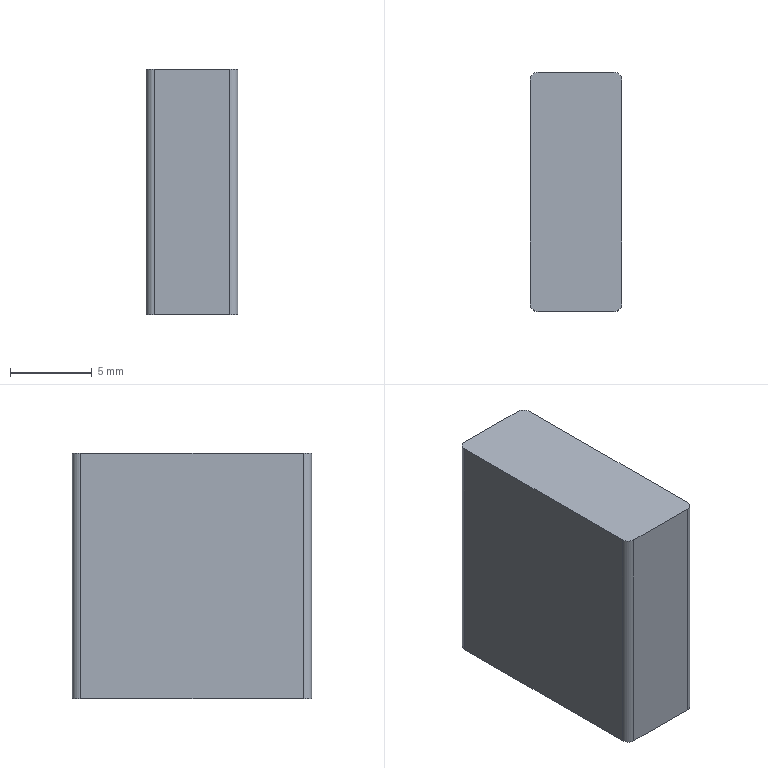Part | NX | features BREP 1 | 1 solid | 10 faces | box 5.6 x 14.6 x 15 mm | volume 1223 mm3 | plane 6 | cylinder 4 | commonest cylinder face diameters 1 x4
STEP:
#1=CARTESIAN_POINT('',(-2.3,7.3,-25.6));
#2=VERTEX_POINT('',#1);
#3=CARTESIAN_POINT('',(-2.8,6.8,-25.6));
#4=VERTEX_POINT('',#3);
#5=CARTESIAN_POINT('',(-2.3,6.8,-25.6));
#6=DIRECTION('',(0.,0.,1.));
#7=DIRECTION('',(1.,0.,0.));
#8=AXIS2_PLACEMENT_3D('',#5,#6,#7);
#9=CIRCLE('',#8,0.5);
#10=EDGE_CURVE('',#2,#4,#9,.T.);
#11=ORIENTED_EDGE('',*,*,#10,.F.);
#12=CARTESIAN_POINT('',(-2.3,7.3,-40.6));
#13=VERTEX_POINT('',#12);
#14=CARTESIAN_POINT('',(-2.3,7.3,-40.6));
#15=DIRECTION('',(0.,0.,1.));
#16=VECTOR('',#15,1000.);
#17=LINE('',#14,#16);
#18=EDGE_CURVE('',#13,#2,#17,.T.);
#19=ORIENTED_EDGE('',*,*,#18,.F.);
#20=CARTESIAN_POINT('',(-2.8,6.8,-40.6));
#21=VERTEX_POINT('',#20);
#22=CARTESIAN_POINT('',(-2.3,6.8,-40.6));
#23=DIRECTION('',(0.,0.,1.));
#24=DIRECTION('',(1.,0.,0.));
#25=AXIS2_PLACEMENT_3D('',#22,#23,#24);
#26=CIRCLE('',#25,0.5);
#27=EDGE_CURVE('',#13,#21,#26,.T.);
#28=ORIENTED_EDGE('',*,*,#27,.T.);
#29=CARTESIAN_POINT('',(-2.8,6.8,-40.6));
#30=DIRECTION('',(0.,0.,1.));
#31=VECTOR('',#30,1000.);
#32=LINE('',#29,#31);
#33=EDGE_CURVE('',#21,#4,#32,.T.);
#34=ORIENTED_EDGE('',*,*,#33,.T.);
#35=EDGE_LOOP('',(#11,#19,#28,#34));
#36=FACE_BOUND('',#35,.T.);
#37=CARTESIAN_POINT('',(-2.3,6.8,-40.6));
#38=DIRECTION('',(0.,0.,1.));
#39=DIRECTION('',(-1.,0.,0.));
#40=AXIS2_PLACEMENT_3D('',#37,#38,#39);
#41=CYLINDRICAL_SURFACE('',#40,0.5);
#42=ADVANCED_FACE('',(#36),#41,.T.);
#43=CARTESIAN_POINT('',(-2.8,-6.8,-25.6));
#44=VERTEX_POINT('',#43);
#45=CARTESIAN_POINT('',(-2.8,-6.8,-25.6));
#46=DIRECTION('',(0.,1.,0.));
#47=VECTOR('',#46,1000.);
#48=LINE('',#45,#47);
#49=EDGE_CURVE('',#44,#4,#48,.T.);
#50=ORIENTED_EDGE('',*,*,#49,.T.);
#51=ORIENTED_EDGE('',*,*,#33,.F.);
#52=CARTESIAN_POINT('',(-2.8,-6.8,-40.6));
#53=VERTEX_POINT('',#52);
#54=CARTESIAN_POINT('',(-2.8,-6.8,-40.6));
#55=DIRECTION('',(0.,1.,0.));
#56=VECTOR('',#55,1000.);
#57=LINE('',#54,#56);
#58=EDGE_CURVE('',#53,#21,#57,.T.);
#59=ORIENTED_EDGE('',*,*,#58,.F.);
#60=CARTESIAN_POINT('',(-2.8,-6.8,-40.6));
#61=DIRECTION('',(0.,0.,1.));
#62=VECTOR('',#61,1000.);
#63=LINE('',#60,#62);
#64=EDGE_CURVE('',#53,#44,#63,.T.);
#65=ORIENTED_EDGE('',*,*,#64,.T.);
#66=EDGE_LOOP('',(#50,#51,#59,#65));
#67=FACE_BOUND('',#66,.T.);
#68=CARTESIAN_POINT('',(-2.8,-6.8,-40.6));
#69=DIRECTION('',(1.,0.,0.));
#70=DIRECTION('',(0.,-1.,0.));
#71=AXIS2_PLACEMENT_3D('',#68,#69,#70);
#72=PLANE('',#71);
#73=ADVANCED_FACE('',(#67),#72,.F.);
#74=CARTESIAN_POINT('',(-2.3,-7.3,-25.6));
#75=VERTEX_POINT('',#74);
#76=CARTESIAN_POINT('',(-2.3,-6.8,-25.6));
#77=DIRECTION('',(0.,0.,1.));
#78=DIRECTION('',(1.,0.,0.));
#79=AXIS2_PLACEMENT_3D('',#76,#77,#78);
#80=CIRCLE('',#79,0.5);
#81=EDGE_CURVE('',#44,#75,#80,.T.);
#82=ORIENTED_EDGE('',*,*,#81,.F.);
#83=ORIENTED_EDGE('',*,*,#64,.F.);
#84=CARTESIAN_POINT('',(-2.3,-7.3,-40.6));
#85=VERTEX_POINT('',#84);
#86=CARTESIAN_POINT('',(-2.3,-6.8,-40.6));
#87=DIRECTION('',(0.,0.,1.));
#88=DIRECTION('',(1.,0.,0.));
#89=AXIS2_PLACEMENT_3D('',#86,#87,#88);
#90=CIRCLE('',#89,0.5);
#91=EDGE_CURVE('',#53,#85,#90,.T.);
#92=ORIENTED_EDGE('',*,*,#91,.T.);
#93=CARTESIAN_POINT('',(-2.3,-7.3,-40.6));
#94=DIRECTION('',(0.,0.,1.));
#95=VECTOR('',#94,1000.);
#96=LINE('',#93,#95);
#97=EDGE_CURVE('',#85,#75,#96,.T.);
#98=ORIENTED_EDGE('',*,*,#97,.T.);
#99=EDGE_LOOP('',(#82,#83,#92,#98));
#100=FACE_BOUND('',#99,.T.);
#101=CARTESIAN_POINT('',(-2.3,-6.8,-40.6));
#102=DIRECTION('',(0.,0.,1.));
#103=DIRECTION('',(-1.,0.,0.));
#104=AXIS2_PLACEMENT_3D('',#101,#102,#103);
#105=CYLINDRICAL_SURFACE('',#104,0.5);
#106=ADVANCED_FACE('',(#100),#105,.T.);
#107=CARTESIAN_POINT('',(2.3,-7.3,-25.6));
#108=VERTEX_POINT('',#107);
#109=CARTESIAN_POINT('',(2.3,-7.3,-25.6));
#110=DIRECTION('',(-1.,0.,0.));
#111=VECTOR('',#110,1000.);
#112=LINE('',#109,#111);
#113=EDGE_CURVE('',#108,#75,#112,.T.);
#114=ORIENTED_EDGE('',*,*,#113,.T.);
#115=ORIENTED_EDGE('',*,*,#97,.F.);
#116=CARTESIAN_POINT('',(2.3,-7.3,-40.6));
#117=VERTEX_POINT('',#116);
#118=CARTESIAN_POINT('',(2.3,-7.3,-40.6));
#119=DIRECTION('',(-1.,0.,0.));
#120=VECTOR('',#119,1000.);
#121=LINE('',#118,#120);
#122=EDGE_CURVE('',#117,#85,#121,.T.);
#123=ORIENTED_EDGE('',*,*,#122,.F.);
#124=CARTESIAN_POINT('',(2.3,-7.3,-40.6));
#125=DIRECTION('',(0.,0.,1.));
#126=VECTOR('',#125,1000.);
#127=LINE('',#124,#126);
#128=EDGE_CURVE('',#117,#108,#127,.T.);
#129=ORIENTED_EDGE('',*,*,#128,.T.);
#130=EDGE_LOOP('',(#114,#115,#123,#129));
#131=FACE_BOUND('',#130,.T.);
#132=CARTESIAN_POINT('',(2.3,-7.3,-40.6));
#133=DIRECTION('',(0.,1.,0.));
#134=DIRECTION('',(0.,0.,-1.));
#135=AXIS2_PLACEMENT_3D('',#132,#133,#134);
#136=PLANE('',#135);
#137=ADVANCED_FACE('',(#131),#136,.F.);
#138=CARTESIAN_POINT('',(2.8,-6.8,-25.6));
#139=VERTEX_POINT('',#138);
#140=CARTESIAN_POINT('',(2.3,-6.8,-25.6));
#141=DIRECTION('',(0.,0.,1.));
#142=DIRECTION('',(1.,0.,0.));
#143=AXIS2_PLACEMENT_3D('',#140,#141,#142);
#144=CIRCLE('',#143,0.5);
#145=EDGE_CURVE('',#108,#139,#144,.T.);
#146=ORIENTED_EDGE('',*,*,#145,.F.);
#147=ORIENTED_EDGE('',*,*,#128,.F.);
#148=CARTESIAN_POINT('',(2.8,-6.8,-40.6));
#149=VERTEX_POINT('',#148);
#150=CARTESIAN_POINT('',(2.3,-6.8,-40.6));
#151=DIRECTION('',(0.,0.,1.));
#152=DIRECTION('',(1.,0.,0.));
#153=AXIS2_PLACEMENT_3D('',#150,#151,#152);
#154=CIRCLE('',#153,0.5);
#155=EDGE_CURVE('',#117,#149,#154,.T.);
#156=ORIENTED_EDGE('',*,*,#155,.T.);
#157=CARTESIAN_POINT('',(2.8,-6.8,-40.6));
#158=DIRECTION('',(0.,0.,1.));
#159=VECTOR('',#158,1000.);
#160=LINE('',#157,#159);
#161=EDGE_CURVE('',#149,#139,#160,.T.);
#162=ORIENTED_EDGE('',*,*,#161,.T.);
#163=EDGE_LOOP('',(#146,#147,#156,#162));
#164=FACE_BOUND('',#163,.T.);
#165=CARTESIAN_POINT('',(2.3,-6.8,-40.6));
#166=DIRECTION('',(0.,0.,1.));
#167=DIRECTION('',(-1.,0.,0.));
#168=AXIS2_PLACEMENT_3D('',#165,#166,#167);
#169=CYLINDRICAL_SURFACE('',#168,0.5);
#170=ADVANCED_FACE('',(#164),#169,.T.);
#171=CARTESIAN_POINT('',(2.8,6.8,-25.6));
#172=VERTEX_POINT('',#171);
#173=CARTESIAN_POINT('',(2.8,6.8,-25.6));
#174=DIRECTION('',(0.,-1.,0.));
#175=VECTOR('',#174,1000.);
#176=LINE('',#173,#175);
#177=EDGE_CURVE('',#172,#139,#176,.T.);
#178=ORIENTED_EDGE('',*,*,#177,.T.);
#179=ORIENTED_EDGE('',*,*,#161,.F.);
#180=CARTESIAN_POINT('',(2.8,6.8,-40.6));
#181=VERTEX_POINT('',#180);
#182=CARTESIAN_POINT('',(2.8,6.8,-40.6));
#183=DIRECTION('',(0.,-1.,0.));
#184=VECTOR('',#183,1000.);
#185=LINE('',#182,#184);
#186=EDGE_CURVE('',#181,#149,#185,.T.);
#187=ORIENTED_EDGE('',*,*,#186,.F.);
#188=CARTESIAN_POINT('',(2.8,6.8,-40.6));
#189=DIRECTION('',(0.,0.,1.));
#190=VECTOR('',#189,1000.);
#191=LINE('',#188,#190);
#192=EDGE_CURVE('',#181,#172,#191,.T.);
#193=ORIENTED_EDGE('',*,*,#192,.T.);
#194=EDGE_LOOP('',(#178,#179,#187,#193));
#195=FACE_BOUND('',#194,.T.);
#196=CARTESIAN_POINT('',(2.8,6.8,-40.6));
#197=DIRECTION('',(-1.,0.,0.));
#198=DIRECTION('',(0.,1.,0.));
#199=AXIS2_PLACEMENT_3D('',#196,#197,#198);
#200=PLANE('',#199);
#201=ADVANCED_FACE('',(#195),#200,.F.);
#202=CARTESIAN_POINT('',(2.3,7.3,-25.6));
#203=VERTEX_POINT('',#202);
#204=CARTESIAN_POINT('',(2.3,6.8,-25.6));
#205=DIRECTION('',(0.,0.,1.));
#206=DIRECTION('',(1.,0.,0.));
#207=AXIS2_PLACEMENT_3D('',#204,#205,#206);
#208=CIRCLE('',#207,0.5);
#209=EDGE_CURVE('',#172,#203,#208,.T.);
#210=ORIENTED_EDGE('',*,*,#209,.F.);
#211=ORIENTED_EDGE('',*,*,#192,.F.);
#212=CARTESIAN_POINT('',(2.3,7.3,-40.6));
#213=VERTEX_POINT('',#212);
#214=CARTESIAN_POINT('',(2.3,6.8,-40.6));
#215=DIRECTION('',(0.,0.,1.));
#216=DIRECTION('',(1.,0.,0.));
#217=AXIS2_PLACEMENT_3D('',#214,#215,#216);
#218=CIRCLE('',#217,0.5);
#219=EDGE_CURVE('',#181,#213,#218,.T.);
#220=ORIENTED_EDGE('',*,*,#219,.T.);
#221=CARTESIAN_POINT('',(2.3,7.3,-40.6));
#222=DIRECTION('',(0.,0.,1.));
#223=VECTOR('',#222,1000.);
#224=LINE('',#221,#223);
#225=EDGE_CURVE('',#213,#203,#224,.T.);
#226=ORIENTED_EDGE('',*,*,#225,.T.);
#227=EDGE_LOOP('',(#210,#211,#220,#226));
#228=FACE_BOUND('',#227,.T.);
#229=CARTESIAN_POINT('',(2.3,6.8,-40.6));
#230=DIRECTION('',(0.,0.,1.));
#231=DIRECTION('',(-1.,0.,0.));
#232=AXIS2_PLACEMENT_3D('',#229,#230,#231);
#233=CYLINDRICAL_SURFACE('',#232,0.5);
#234=ADVANCED_FACE('',(#228),#233,.T.);
#235=CARTESIAN_POINT('',(-2.3,7.3,-25.6));
#236=DIRECTION('',(1.,0.,0.));
#237=VECTOR('',#236,1000.);
#238=LINE('',#235,#237);
#239=EDGE_CURVE('',#2,#203,#238,.T.);
#240=ORIENTED_EDGE('',*,*,#239,.T.);
#241=ORIENTED_EDGE('',*,*,#225,.F.);
#242=CARTESIAN_POINT('',(-2.3,7.3,-40.6));
#243=DIRECTION('',(1.,0.,0.));
#244=VECTOR('',#243,1000.);
#245=LINE('',#242,#244);
#246=EDGE_CURVE('',#13,#213,#245,.T.);
#247=ORIENTED_EDGE('',*,*,#246,.F.);
#248=ORIENTED_EDGE('',*,*,#18,.T.);
#249=EDGE_LOOP('',(#240,#241,#247,#248));
#250=FACE_BOUND('',#249,.T.);
#251=CARTESIAN_POINT('',(-2.3,7.3,-40.6));
#252=DIRECTION('',(0.,-1.,0.));
#253=DIRECTION('',(0.,0.,1.));
#254=AXIS2_PLACEMENT_3D('',#251,#252,#253);
#255=PLANE('',#254);
#256=ADVANCED_FACE('',(#250),#255,.F.);
#257=ORIENTED_EDGE('',*,*,#27,.F.);
#258=ORIENTED_EDGE('',*,*,#246,.T.);
#259=ORIENTED_EDGE('',*,*,#219,.F.);
#260=ORIENTED_EDGE('',*,*,#186,.T.);
#261=ORIENTED_EDGE('',*,*,#155,.F.);
#262=ORIENTED_EDGE('',*,*,#122,.T.);
#263=ORIENTED_EDGE('',*,*,#91,.F.);
#264=ORIENTED_EDGE('',*,*,#58,.T.);
#265=EDGE_LOOP('',(#257,#258,#259,#260,#261,#262,#263,#264));
#266=FACE_BOUND('',#265,.T.);
#267=CARTESIAN_POINT('',(-2.3,6.8,-40.6));
#268=DIRECTION('',(0.,0.,1.));
#269=DIRECTION('',(-1.,0.,0.));
#270=AXIS2_PLACEMENT_3D('',#267,#268,#269);
#271=PLANE('',#270);
#272=ADVANCED_FACE('',(#266),#271,.F.);
#273=ORIENTED_EDGE('',*,*,#10,.T.);
#274=ORIENTED_EDGE('',*,*,#49,.F.);
#275=ORIENTED_EDGE('',*,*,#81,.T.);
#276=ORIENTED_EDGE('',*,*,#113,.F.);
#277=ORIENTED_EDGE('',*,*,#145,.T.);
#278=ORIENTED_EDGE('',*,*,#177,.F.);
#279=ORIENTED_EDGE('',*,*,#209,.T.);
#280=ORIENTED_EDGE('',*,*,#239,.F.);
#281=EDGE_LOOP('',(#273,#274,#275,#276,#277,#278,#279,#280));
#282=FACE_BOUND('',#281,.T.);
#283=CARTESIAN_POINT('',(-2.3,6.8,-25.6));
#284=DIRECTION('',(0.,0.,1.));
#285=DIRECTION('',(-1.,0.,0.));
#286=AXIS2_PLACEMENT_3D('',#283,#284,#285);
#287=PLANE('',#286);
#288=ADVANCED_FACE('',(#282),#287,.T.);
#289=CLOSED_SHELL('',(#42,#73,#106,#137,#170,#201,#234,#256,#272,#288));
#290=MANIFOLD_SOLID_BREP('',#289);
#291=(LENGTH_UNIT()NAMED_UNIT(*)SI_UNIT(.MILLI.,.METRE.));
#292=UNCERTAINTY_MEASURE_WITH_UNIT(LENGTH_MEASURE(0.00001),#291,'','');
#293=(NAMED_UNIT(*)PLANE_ANGLE_UNIT()SI_UNIT($,.RADIAN.));
#294=(NAMED_UNIT(*)SI_UNIT($,.STERADIAN.)SOLID_ANGLE_UNIT());
#295=(GEOMETRIC_REPRESENTATION_CONTEXT(3)GLOBAL_UNCERTAINTY_ASSIGNED_CONTEXT((#292))GLOBAL_UNIT_ASSIGNED_CONTEXT((#291,#293,#294))REPRESENTATION_CONTEXT('',''));
#296=ADVANCED_BREP_SHAPE_REPRESENTATION('',(#290),#295);